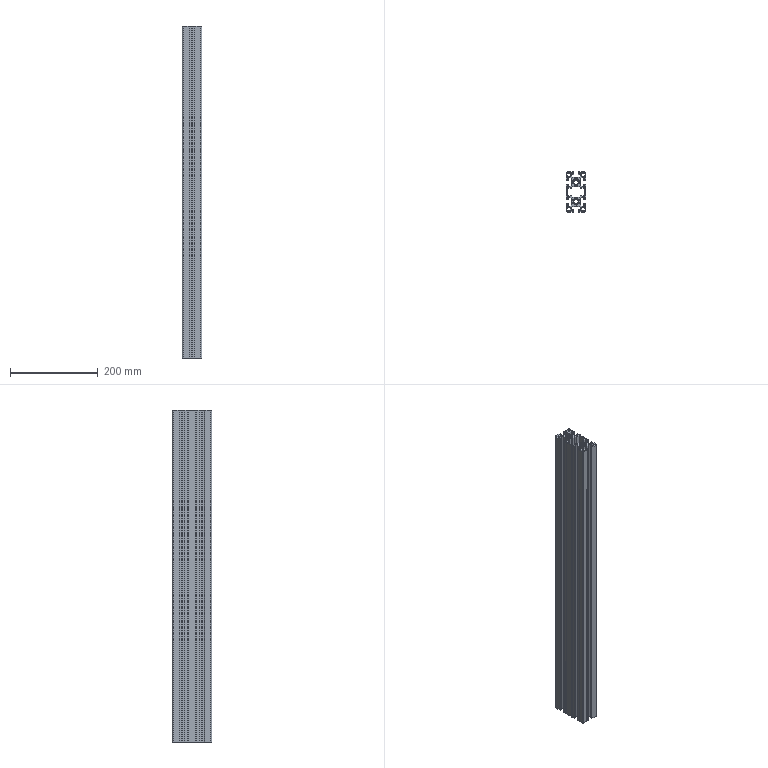Part | STEP file | PN_0020 | 1 solid | 468 faces | box 45 x 90 x 757.5 mm | volume 985388 mm3 | cylinder 262 | plane 206 | commonest cylinder face diameters 1 x116 0.6 x56 2 x40 10.2 x18 16 x16 0.4 x12